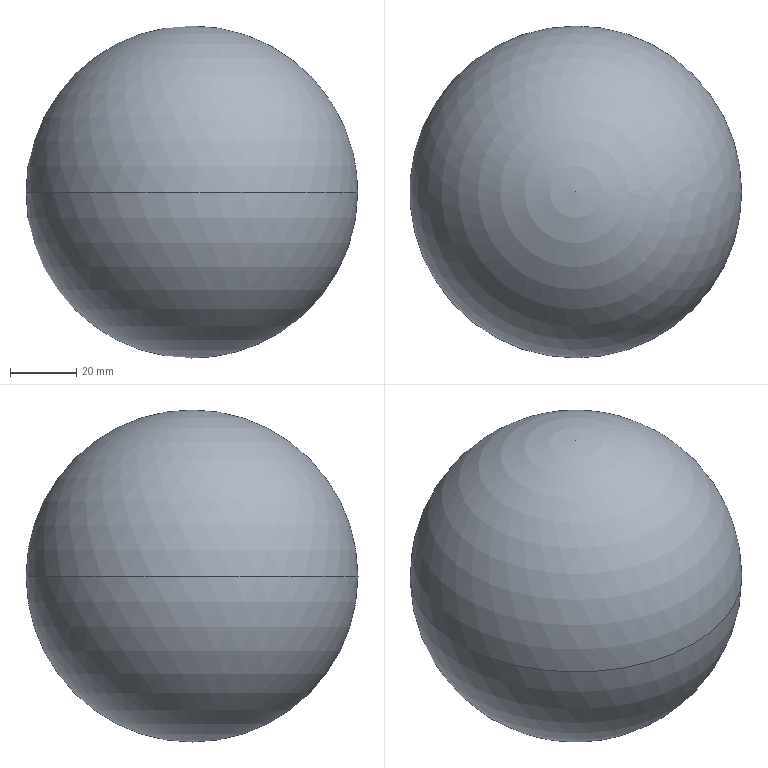Part | SolidWorks | features Revolution 1 | 1 solid | 2 faces | box 100 x 100 x 100 mm | volume 523599 mm3 | sphere 2
STEP:
#1=CARTESIAN_POINT('',(0.,-50.,0.));
#2=VERTEX_POINT('',#1);
#3=CARTESIAN_POINT('',(0.,50.,0.));
#4=VERTEX_POINT('',#3);
#5=CARTESIAN_POINT('',(0.,0.,0.));
#6=DIRECTION('',(0.,0.,1.));
#7=DIRECTION('',(1.,0.,0.));
#8=AXIS2_PLACEMENT_3D('',#5,#6,#7);
#9=CIRCLE('',#8,50.);
#10=EDGE_CURVE('',#2,#4,#9,.T.);
#11=ORIENTED_EDGE('',*,*,#10,.F.);
#12=CARTESIAN_POINT('',(0.,0.,0.));
#13=DIRECTION('',(0.,0.,-1.));
#14=DIRECTION('',(-1.,0.,0.));
#15=AXIS2_PLACEMENT_3D('',#12,#13,#14);
#16=CIRCLE('',#15,50.);
#17=EDGE_CURVE('',#2,#4,#16,.T.);
#18=ORIENTED_EDGE('',*,*,#17,.T.);
#19=EDGE_LOOP('',(#11,#18));
#20=FACE_OUTER_BOUND('',#19,.T.);
#21=CARTESIAN_POINT('',(0.,0.,0.));
#22=DIRECTION('',(0.,0.,-1.));
#23=DIRECTION('',(1.,0.,0.));
#24=AXIS2_PLACEMENT_3D('',#21,#22,#23);
#25=SPHERICAL_SURFACE('',#24,50.);
#26=ADVANCED_FACE('',(#20),#25,.T.);
#27=ORIENTED_EDGE('',*,*,#17,.F.);
#28=ORIENTED_EDGE('',*,*,#10,.T.);
#29=EDGE_LOOP('',(#27,#28));
#30=FACE_OUTER_BOUND('',#29,.T.);
#31=CARTESIAN_POINT('',(0.,0.,0.));
#32=DIRECTION('',(0.,0.,-1.));
#33=DIRECTION('',(1.,0.,0.));
#34=AXIS2_PLACEMENT_3D('',#31,#32,#33);
#35=SPHERICAL_SURFACE('',#34,50.);
#36=ADVANCED_FACE('',(#30),#35,.T.);
#37=CLOSED_SHELL('',(#26,#36));
#38=MANIFOLD_SOLID_BREP('',#37);
#39=CARTESIAN_POINT('',(0.,0.,0.));
#40=DIRECTION('',(0.,0.,1.));
#41=DIRECTION('',(1.,0.,0.));
#42=AXIS2_PLACEMENT_3D('',#39,#40,#41);
#43=(LENGTH_UNIT()NAMED_UNIT(*)SI_UNIT(.MILLI.,.METRE.));
#44=UNCERTAINTY_MEASURE_WITH_UNIT(LENGTH_MEASURE(0.00001),#43,'','');
#45=(NAMED_UNIT(*)PLANE_ANGLE_UNIT()SI_UNIT($,.RADIAN.));
#46=(NAMED_UNIT(*)SI_UNIT($,.STERADIAN.)SOLID_ANGLE_UNIT());
#47=(GEOMETRIC_REPRESENTATION_CONTEXT(3)GLOBAL_UNCERTAINTY_ASSIGNED_CONTEXT((#44))GLOBAL_UNIT_ASSIGNED_CONTEXT((#43,#45,#46))REPRESENTATION_CONTEXT('',''));
#48=ADVANCED_BREP_SHAPE_REPRESENTATION('',(#38,#42),#47);